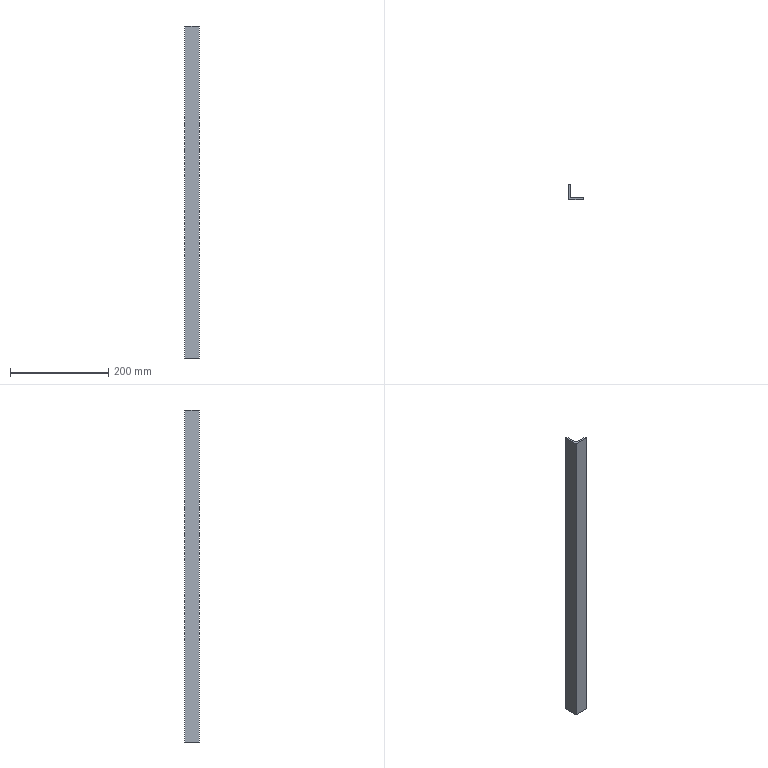Part | SolidWorks | features Extrusion 1 | 1 solid | 11 faces | box 30 x 30 x 675 mm | volume 118069 mm3 | plane 8 | cylinder 3 | commonest cylinder face diameters 2 x2 9 x1
STEP:
#1=CARTESIAN_POINT('',(2.,30.,-337.5));
#2=VERTEX_POINT('',#1);
#3=CARTESIAN_POINT('',(3.,29.,-337.5));
#4=VERTEX_POINT('',#3);
#5=CARTESIAN_POINT('',(2.,29.,-337.5));
#6=DIRECTION('',(0.,0.,-1.));
#7=DIRECTION('',(-1.,0.,0.));
#8=AXIS2_PLACEMENT_3D('',#5,#6,#7);
#9=CIRCLE('',#8,1.);
#10=EDGE_CURVE('',#2,#4,#9,.T.);
#11=ORIENTED_EDGE('',*,*,#10,.F.);
#12=CARTESIAN_POINT('',(2.,30.,337.5));
#13=VERTEX_POINT('',#12);
#14=CARTESIAN_POINT('',(2.,30.,337.5));
#15=DIRECTION('',(0.,0.,-1.));
#16=VECTOR('',#15,1000.);
#17=LINE('',#14,#16);
#18=EDGE_CURVE('',#13,#2,#17,.T.);
#19=ORIENTED_EDGE('',*,*,#18,.F.);
#20=CARTESIAN_POINT('',(3.,29.,337.5));
#21=VERTEX_POINT('',#20);
#22=CARTESIAN_POINT('',(2.,29.,337.5));
#23=DIRECTION('',(0.,0.,-1.));
#24=DIRECTION('',(-1.,0.,0.));
#25=AXIS2_PLACEMENT_3D('',#22,#23,#24);
#26=CIRCLE('',#25,1.);
#27=EDGE_CURVE('',#13,#21,#26,.T.);
#28=ORIENTED_EDGE('',*,*,#27,.T.);
#29=CARTESIAN_POINT('',(3.,29.,337.5));
#30=DIRECTION('',(0.,0.,-1.));
#31=VECTOR('',#30,1000.);
#32=LINE('',#29,#31);
#33=EDGE_CURVE('',#21,#4,#32,.T.);
#34=ORIENTED_EDGE('',*,*,#33,.T.);
#35=EDGE_LOOP('',(#11,#19,#28,#34));
#36=FACE_OUTER_BOUND('',#35,.T.);
#37=CARTESIAN_POINT('',(2.,29.,337.5));
#38=DIRECTION('',(0.,0.,-1.));
#39=DIRECTION('',(-1.,0.,0.));
#40=AXIS2_PLACEMENT_3D('',#37,#38,#39);
#41=CYLINDRICAL_SURFACE('',#40,1.);
#42=ADVANCED_FACE('',(#36),#41,.T.);
#43=CARTESIAN_POINT('',(0.,30.,-337.5));
#44=VERTEX_POINT('',#43);
#45=CARTESIAN_POINT('',(0.,30.,-337.5));
#46=DIRECTION('',(1.,0.,0.));
#47=VECTOR('',#46,1000.);
#48=LINE('',#45,#47);
#49=EDGE_CURVE('',#44,#2,#48,.T.);
#50=ORIENTED_EDGE('',*,*,#49,.F.);
#51=CARTESIAN_POINT('',(0.,30.,337.5));
#52=VERTEX_POINT('',#51);
#53=CARTESIAN_POINT('',(0.,30.,337.5));
#54=DIRECTION('',(0.,0.,-1.));
#55=VECTOR('',#54,1000.);
#56=LINE('',#53,#55);
#57=EDGE_CURVE('',#52,#44,#56,.T.);
#58=ORIENTED_EDGE('',*,*,#57,.F.);
#59=CARTESIAN_POINT('',(0.,30.,337.5));
#60=DIRECTION('',(1.,0.,0.));
#61=VECTOR('',#60,1000.);
#62=LINE('',#59,#61);
#63=EDGE_CURVE('',#52,#13,#62,.T.);
#64=ORIENTED_EDGE('',*,*,#63,.T.);
#65=ORIENTED_EDGE('',*,*,#18,.T.);
#66=EDGE_LOOP('',(#50,#58,#64,#65));
#67=FACE_OUTER_BOUND('',#66,.T.);
#68=CARTESIAN_POINT('',(0.,30.,337.5));
#69=DIRECTION('',(0.,1.,0.));
#70=DIRECTION('',(0.,0.,1.));
#71=AXIS2_PLACEMENT_3D('',#68,#69,#70);
#72=PLANE('',#71);
#73=ADVANCED_FACE('',(#67),#72,.T.);
#74=CARTESIAN_POINT('',(0.,0.,-337.5));
#75=VERTEX_POINT('',#74);
#76=CARTESIAN_POINT('',(0.,0.,-337.5));
#77=DIRECTION('',(0.,1.,0.));
#78=VECTOR('',#77,1000.);
#79=LINE('',#76,#78);
#80=EDGE_CURVE('',#75,#44,#79,.T.);
#81=ORIENTED_EDGE('',*,*,#80,.F.);
#82=CARTESIAN_POINT('',(0.,0.,337.5));
#83=VERTEX_POINT('',#82);
#84=CARTESIAN_POINT('',(0.,0.,337.5));
#85=DIRECTION('',(0.,0.,-1.));
#86=VECTOR('',#85,1000.);
#87=LINE('',#84,#86);
#88=EDGE_CURVE('',#83,#75,#87,.T.);
#89=ORIENTED_EDGE('',*,*,#88,.F.);
#90=CARTESIAN_POINT('',(0.,0.,337.5));
#91=DIRECTION('',(0.,1.,0.));
#92=VECTOR('',#91,1000.);
#93=LINE('',#90,#92);
#94=EDGE_CURVE('',#83,#52,#93,.T.);
#95=ORIENTED_EDGE('',*,*,#94,.T.);
#96=ORIENTED_EDGE('',*,*,#57,.T.);
#97=EDGE_LOOP('',(#81,#89,#95,#96));
#98=FACE_OUTER_BOUND('',#97,.T.);
#99=CARTESIAN_POINT('',(0.,0.,337.5));
#100=DIRECTION('',(-1.,0.,0.));
#101=DIRECTION('',(0.,0.,1.));
#102=AXIS2_PLACEMENT_3D('',#99,#100,#101);
#103=PLANE('',#102);
#104=ADVANCED_FACE('',(#98),#103,.T.);
#105=CARTESIAN_POINT('',(30.,0.,-337.5));
#106=VERTEX_POINT('',#105);
#107=CARTESIAN_POINT('',(30.,0.,-337.5));
#108=DIRECTION('',(-1.,0.,0.));
#109=VECTOR('',#108,1000.);
#110=LINE('',#107,#109);
#111=EDGE_CURVE('',#106,#75,#110,.T.);
#112=ORIENTED_EDGE('',*,*,#111,.F.);
#113=CARTESIAN_POINT('',(30.,0.,337.5));
#114=VERTEX_POINT('',#113);
#115=CARTESIAN_POINT('',(30.,0.,337.5));
#116=DIRECTION('',(0.,0.,-1.));
#117=VECTOR('',#116,1000.);
#118=LINE('',#115,#117);
#119=EDGE_CURVE('',#114,#106,#118,.T.);
#120=ORIENTED_EDGE('',*,*,#119,.F.);
#121=CARTESIAN_POINT('',(30.,0.,337.5));
#122=DIRECTION('',(-1.,0.,0.));
#123=VECTOR('',#122,1000.);
#124=LINE('',#121,#123);
#125=EDGE_CURVE('',#114,#83,#124,.T.);
#126=ORIENTED_EDGE('',*,*,#125,.T.);
#127=ORIENTED_EDGE('',*,*,#88,.T.);
#128=EDGE_LOOP('',(#112,#120,#126,#127));
#129=FACE_OUTER_BOUND('',#128,.T.);
#130=CARTESIAN_POINT('',(30.,0.,337.5));
#131=DIRECTION('',(0.,-1.,0.));
#132=DIRECTION('',(0.,0.,-1.));
#133=AXIS2_PLACEMENT_3D('',#130,#131,#132);
#134=PLANE('',#133);
#135=ADVANCED_FACE('',(#129),#134,.T.);
#136=CARTESIAN_POINT('',(30.,2.,-337.5));
#137=VERTEX_POINT('',#136);
#138=CARTESIAN_POINT('',(30.,0.,-337.5));
#139=DIRECTION('',(0.,1.,0.));
#140=VECTOR('',#139,1000.);
#141=LINE('',#138,#140);
#142=EDGE_CURVE('',#106,#137,#141,.T.);
#143=ORIENTED_EDGE('',*,*,#142,.T.);
#144=CARTESIAN_POINT('',(30.,2.,337.5));
#145=VERTEX_POINT('',#144);
#146=CARTESIAN_POINT('',(30.,2.,337.5));
#147=DIRECTION('',(0.,0.,-1.));
#148=VECTOR('',#147,1000.);
#149=LINE('',#146,#148);
#150=EDGE_CURVE('',#145,#137,#149,.T.);
#151=ORIENTED_EDGE('',*,*,#150,.F.);
#152=CARTESIAN_POINT('',(30.,0.,337.5));
#153=DIRECTION('',(0.,1.,0.));
#154=VECTOR('',#153,1000.);
#155=LINE('',#152,#154);
#156=EDGE_CURVE('',#114,#145,#155,.T.);
#157=ORIENTED_EDGE('',*,*,#156,.F.);
#158=ORIENTED_EDGE('',*,*,#119,.T.);
#159=EDGE_LOOP('',(#143,#151,#157,#158));
#160=FACE_OUTER_BOUND('',#159,.T.);
#161=CARTESIAN_POINT('',(30.,0.,337.5));
#162=DIRECTION('',(-1.,0.,0.));
#163=DIRECTION('',(0.,0.,1.));
#164=AXIS2_PLACEMENT_3D('',#161,#162,#163);
#165=PLANE('',#164);
#166=ADVANCED_FACE('',(#160),#165,.F.);
#167=CARTESIAN_POINT('',(29.,3.,-337.5));
#168=VERTEX_POINT('',#167);
#169=CARTESIAN_POINT('',(29.,2.,-337.5));
#170=DIRECTION('',(0.,0.,1.));
#171=DIRECTION('',(1.,0.,0.));
#172=AXIS2_PLACEMENT_3D('',#169,#170,#171);
#173=CIRCLE('',#172,1.);
#174=EDGE_CURVE('',#137,#168,#173,.T.);
#175=ORIENTED_EDGE('',*,*,#174,.T.);
#176=CARTESIAN_POINT('',(29.,3.,337.5));
#177=VERTEX_POINT('',#176);
#178=CARTESIAN_POINT('',(29.,3.,337.5));
#179=DIRECTION('',(0.,0.,-1.));
#180=VECTOR('',#179,1000.);
#181=LINE('',#178,#180);
#182=EDGE_CURVE('',#177,#168,#181,.T.);
#183=ORIENTED_EDGE('',*,*,#182,.F.);
#184=CARTESIAN_POINT('',(29.,2.,337.5));
#185=DIRECTION('',(0.,0.,1.));
#186=DIRECTION('',(1.,0.,0.));
#187=AXIS2_PLACEMENT_3D('',#184,#185,#186);
#188=CIRCLE('',#187,1.);
#189=EDGE_CURVE('',#145,#177,#188,.T.);
#190=ORIENTED_EDGE('',*,*,#189,.F.);
#191=ORIENTED_EDGE('',*,*,#150,.T.);
#192=EDGE_LOOP('',(#175,#183,#190,#191));
#193=FACE_OUTER_BOUND('',#192,.T.);
#194=CARTESIAN_POINT('',(29.,2.,337.5));
#195=DIRECTION('',(0.,0.,-1.));
#196=DIRECTION('',(-1.,0.,0.));
#197=AXIS2_PLACEMENT_3D('',#194,#195,#196);
#198=CYLINDRICAL_SURFACE('',#197,1.);
#199=ADVANCED_FACE('',(#193),#198,.T.);
#200=CARTESIAN_POINT('',(7.5,3.,-337.5));
#201=VERTEX_POINT('',#200);
#202=CARTESIAN_POINT('',(7.5,3.,-337.5));
#203=DIRECTION('',(1.,0.,0.));
#204=VECTOR('',#203,1000.);
#205=LINE('',#202,#204);
#206=EDGE_CURVE('',#201,#168,#205,.T.);
#207=ORIENTED_EDGE('',*,*,#206,.F.);
#208=CARTESIAN_POINT('',(7.5,3.,337.5));
#209=VERTEX_POINT('',#208);
#210=CARTESIAN_POINT('',(7.5,3.,337.5));
#211=DIRECTION('',(0.,0.,-1.));
#212=VECTOR('',#211,1000.);
#213=LINE('',#210,#212);
#214=EDGE_CURVE('',#209,#201,#213,.T.);
#215=ORIENTED_EDGE('',*,*,#214,.F.);
#216=CARTESIAN_POINT('',(7.5,3.,337.5));
#217=DIRECTION('',(1.,0.,0.));
#218=VECTOR('',#217,1000.);
#219=LINE('',#216,#218);
#220=EDGE_CURVE('',#209,#177,#219,.T.);
#221=ORIENTED_EDGE('',*,*,#220,.T.);
#222=ORIENTED_EDGE('',*,*,#182,.T.);
#223=EDGE_LOOP('',(#207,#215,#221,#222));
#224=FACE_OUTER_BOUND('',#223,.T.);
#225=CARTESIAN_POINT('',(7.5,3.,337.5));
#226=DIRECTION('',(0.,1.,0.));
#227=DIRECTION('',(-1.,0.,0.));
#228=AXIS2_PLACEMENT_3D('',#225,#226,#227);
#229=PLANE('',#228);
#230=ADVANCED_FACE('',(#224),#229,.T.);
#231=CARTESIAN_POINT('',(3.,7.5,-337.5));
#232=VERTEX_POINT('',#231);
#233=CARTESIAN_POINT('',(7.5,7.5,-337.5));
#234=DIRECTION('',(0.,0.,-1.));
#235=DIRECTION('',(-1.,0.,0.));
#236=AXIS2_PLACEMENT_3D('',#233,#234,#235);
#237=CIRCLE('',#236,4.5);
#238=EDGE_CURVE('',#201,#232,#237,.T.);
#239=ORIENTED_EDGE('',*,*,#238,.T.);
#240=CARTESIAN_POINT('',(3.,7.5,337.5));
#241=VERTEX_POINT('',#240);
#242=CARTESIAN_POINT('',(3.,7.5,337.5));
#243=DIRECTION('',(0.,0.,-1.));
#244=VECTOR('',#243,1000.);
#245=LINE('',#242,#244);
#246=EDGE_CURVE('',#241,#232,#245,.T.);
#247=ORIENTED_EDGE('',*,*,#246,.F.);
#248=CARTESIAN_POINT('',(7.5,7.5,337.5));
#249=DIRECTION('',(0.,0.,-1.));
#250=DIRECTION('',(-1.,0.,0.));
#251=AXIS2_PLACEMENT_3D('',#248,#249,#250);
#252=CIRCLE('',#251,4.5);
#253=EDGE_CURVE('',#209,#241,#252,.T.);
#254=ORIENTED_EDGE('',*,*,#253,.F.);
#255=ORIENTED_EDGE('',*,*,#214,.T.);
#256=EDGE_LOOP('',(#239,#247,#254,#255));
#257=FACE_OUTER_BOUND('',#256,.T.);
#258=CARTESIAN_POINT('',(7.5,7.5,337.5));
#259=DIRECTION('',(0.,0.,-1.));
#260=DIRECTION('',(-1.,0.,0.));
#261=AXIS2_PLACEMENT_3D('',#258,#259,#260);
#262=CYLINDRICAL_SURFACE('',#261,4.5);
#263=ADVANCED_FACE('',(#257),#262,.F.);
#264=CARTESIAN_POINT('',(3.,29.,-337.5));
#265=DIRECTION('',(0.,-1.,0.));
#266=VECTOR('',#265,1000.);
#267=LINE('',#264,#266);
#268=EDGE_CURVE('',#4,#232,#267,.T.);
#269=ORIENTED_EDGE('',*,*,#268,.F.);
#270=ORIENTED_EDGE('',*,*,#33,.F.);
#271=CARTESIAN_POINT('',(3.,29.,337.5));
#272=DIRECTION('',(0.,-1.,0.));
#273=VECTOR('',#272,1000.);
#274=LINE('',#271,#273);
#275=EDGE_CURVE('',#21,#241,#274,.T.);
#276=ORIENTED_EDGE('',*,*,#275,.T.);
#277=ORIENTED_EDGE('',*,*,#246,.T.);
#278=EDGE_LOOP('',(#269,#270,#276,#277));
#279=FACE_OUTER_BOUND('',#278,.T.);
#280=CARTESIAN_POINT('',(3.,29.,337.5));
#281=DIRECTION('',(1.,0.,0.));
#282=DIRECTION('',(0.,1.,0.));
#283=AXIS2_PLACEMENT_3D('',#280,#281,#282);
#284=PLANE('',#283);
#285=ADVANCED_FACE('',(#279),#284,.T.);
#286=ORIENTED_EDGE('',*,*,#27,.F.);
#287=ORIENTED_EDGE('',*,*,#63,.F.);
#288=ORIENTED_EDGE('',*,*,#94,.F.);
#289=ORIENTED_EDGE('',*,*,#125,.F.);
#290=ORIENTED_EDGE('',*,*,#156,.T.);
#291=ORIENTED_EDGE('',*,*,#189,.T.);
#292=ORIENTED_EDGE('',*,*,#220,.F.);
#293=ORIENTED_EDGE('',*,*,#253,.T.);
#294=ORIENTED_EDGE('',*,*,#275,.F.);
#295=EDGE_LOOP('',(#286,#287,#288,#289,#290,#291,#292,#293,#294));
#296=FACE_OUTER_BOUND('',#295,.T.);
#297=CARTESIAN_POINT('',(2.,29.,337.5));
#298=DIRECTION('',(0.,0.,-1.));
#299=DIRECTION('',(-1.,0.,0.));
#300=AXIS2_PLACEMENT_3D('',#297,#298,#299);
#301=PLANE('',#300);
#302=ADVANCED_FACE('',(#296),#301,.F.);
#303=ORIENTED_EDGE('',*,*,#10,.T.);
#304=ORIENTED_EDGE('',*,*,#268,.T.);
#305=ORIENTED_EDGE('',*,*,#238,.F.);
#306=ORIENTED_EDGE('',*,*,#206,.T.);
#307=ORIENTED_EDGE('',*,*,#174,.F.);
#308=ORIENTED_EDGE('',*,*,#142,.F.);
#309=ORIENTED_EDGE('',*,*,#111,.T.);
#310=ORIENTED_EDGE('',*,*,#80,.T.);
#311=ORIENTED_EDGE('',*,*,#49,.T.);
#312=EDGE_LOOP('',(#303,#304,#305,#306,#307,#308,#309,#310,#311));
#313=FACE_OUTER_BOUND('',#312,.T.);
#314=CARTESIAN_POINT('',(2.,29.,-337.5));
#315=DIRECTION('',(0.,0.,-1.));
#316=DIRECTION('',(-1.,0.,0.));
#317=AXIS2_PLACEMENT_3D('',#314,#315,#316);
#318=PLANE('',#317);
#319=ADVANCED_FACE('',(#313),#318,.T.);
#320=CLOSED_SHELL('',(#42,#73,#104,#135,#166,#199,#230,#263,#285,#302,#319));
#321=MANIFOLD_SOLID_BREP('',#320);
#322=CARTESIAN_POINT('',(0.,0.,0.));
#323=DIRECTION('',(0.,0.,1.));
#324=DIRECTION('',(1.,0.,0.));
#325=AXIS2_PLACEMENT_3D('',#322,#323,#324);
#326=(LENGTH_UNIT()NAMED_UNIT(*)SI_UNIT(.MILLI.,.METRE.));
#327=UNCERTAINTY_MEASURE_WITH_UNIT(LENGTH_MEASURE(0.00001),#326,'','');
#328=(NAMED_UNIT(*)PLANE_ANGLE_UNIT()SI_UNIT($,.RADIAN.));
#329=(NAMED_UNIT(*)SI_UNIT($,.STERADIAN.)SOLID_ANGLE_UNIT());
#330=(GEOMETRIC_REPRESENTATION_CONTEXT(3)GLOBAL_UNCERTAINTY_ASSIGNED_CONTEXT((#327))GLOBAL_UNIT_ASSIGNED_CONTEXT((#326,#328,#329))REPRESENTATION_CONTEXT('',''));
#331=ADVANCED_BREP_SHAPE_REPRESENTATION('',(#321,#325),#330);